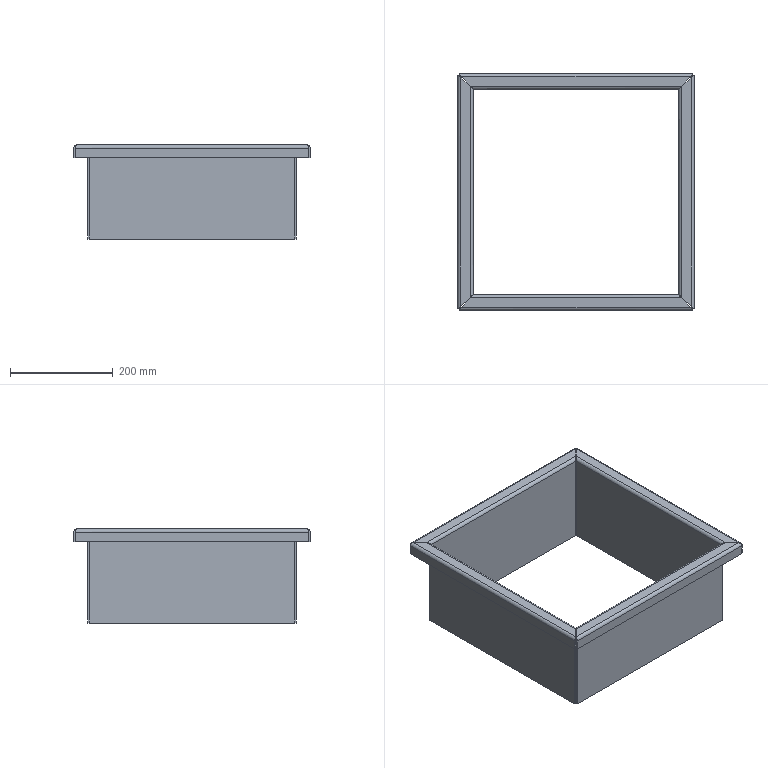Part | SolidWorks | features FlatPattern 4, ICE 1, SMBaseFlange 1, SMMiteredFlange 1, SheetMetal 1 | 4 solids | 88 faces | box 460 x 460 x 183 mm | volume 1117648 mm3 | plane 56 | spline 16 | cylinder 16 | commonest cylinder face diameters 6 x8 12 x8